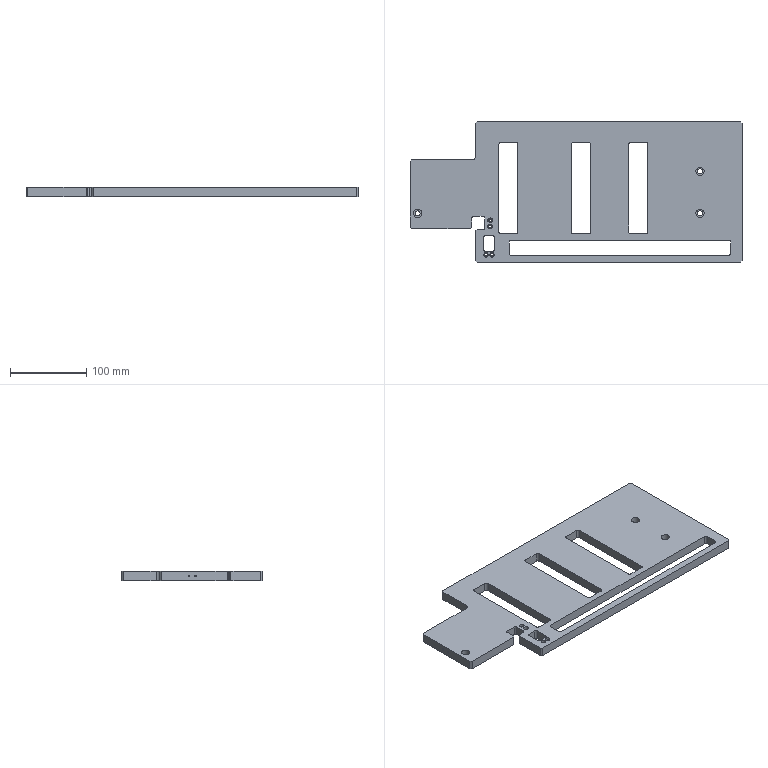NC program | NX | posted with a generic post | part box 435 x 184 x 12 mm
Lines 1793 to 2749 of 10210:
(HOLE_MILLING , TOOL : D6)
N3530 T12 M6
N3532 G54
N3534 G17 G0 G90 X-207.5 Y-28. S9500 M3
N3536 G43 Z30. H12
N3538 Z1.
N3540 G94 G3 X-206.25 Y-29.25 R1.25 F1500.
N3542 X-205. Y-28. R1.25
N3544 X-205. Y-28. Z0.5 I-2.5 J0.
N3546 X-205. Y-28. Z0. I-2.5 J0.
N3548 X-205. Y-28. Z-0.5 I-2.5 J0.
N3550 X-205. Y-28. Z-1. I-2.5 J0.
N3552 X-205. Y-28. Z-1.5 I-2.5 J0.
N3554 X-205. Y-28. Z-2. I-2.5 J0.
N3556 X-205. Y-28. Z-2.5 I-2.5 J0.
N3558 X-205. Y-28. Z-3. I-2.5 J0.
N3560 X-205. Y-28. Z-3.5 I-2.5 J0.
N3562 X-205. Y-28. Z-4. I-2.5 J0.
N3564 X-205. Y-28. Z-4.5 I-2.5 J0.
N3566 X-205. Y-28. Z-5. I-2.5 J0.
N3568 X-205. Y-28. Z-5.5 I-2.5 J0.
N3570 X-205. Y-28. Z-6. I-2.5 J0.
N3572 X-205. Y-28. Z-6.5 I-2.5 J0.
N3574 X-205. Y-28. Z-7. I-2.5 J0.
N3576 X-207.5 Y-25.5 R2.5
N3578 X-205. Y-28. R-2.5
N3580 X-206.25 Y-26.75 R1.25
N3582 X-207.5 Y-28. R1.25
N3584 G0 Z30.
N3586 X162.5
N3588 Z1.
N3590 G3 X163.75 Y-29.25 R1.25
N3592 X165. Y-28. R1.25
N3594 X165. Y-28. Z0.5 I-2.5 J0.
N3596 X165. Y-28. Z0. I-2.5 J0.
N3598 X165. Y-28. Z-0.5 I-2.5 J0.
N3600 X165. Y-28. Z-1. I-2.5 J0.
N3602 X165. Y-28. Z-1.5 I-2.5 J0.
N3604 X165. Y-28. Z-2. I-2.5 J0.
N3606 X165. Y-28. Z-2.5 I-2.5 J0.
N3608 X165. Y-28. Z-3. I-2.5 J0.
N3610 X165. Y-28. Z-3.5 I-2.5 J0.
N3612 X165. Y-28. Z-4. I-2.5 J0.
N3614 X165. Y-28. Z-4.5 I-2.5 J0.
N3616 X165. Y-28. Z-5. I-2.5 J0.
N3618 X165. Y-28. Z-5.5 I-2.5 J0.
N3620 X165. Y-28. Z-6. I-2.5 J0.
N3622 X165. Y-28. Z-6.5 I-2.5 J0.
N3624 X165. Y-28. Z-7. I-2.5 J0.
N3626 X162.5 Y-25.5 R2.5
N3628 X165. Y-28. R-2.5
N3630 X163.75 Y-26.75 R1.25
N3632 X162.5 Y-28. R1.25
N3634 G0 Z30.
N3636 Y27.
N3638 Z1.
N3640 G3 X163.75 Y25.75 R1.25
N3642 X165. Y27. R1.25
N3644 X165. Y27. Z0.5 I-2.5 J0.
N3646 X165. Y27. Z0. I-2.5 J0.
N3648 X165. Y27. Z-0.5 I-2.5 J0.
N3650 X165. Y27. Z-1. I-2.5 J0.
N3652 X165. Y27. Z-1.5 I-2.5 J0.
N3654 X165. Y27. Z-2. I-2.5 J0.
N3656 X165. Y27. Z-2.5 I-2.5 J0.
N3658 X165. Y27. Z-3. I-2.5 J0.
N3660 X165. Y27. Z-3.5 I-2.5 J0.
N3662 X165. Y27. Z-4. I-2.5 J0.
N3664 X165. Y27. Z-4.5 I-2.5 J0.
N3666 X165. Y27. Z-5. I-2.5 J0.
N3668 X165. Y27. Z-5.5 I-2.5 J0.
N3670 X165. Y27. Z-6. I-2.5 J0.
N3672 X165. Y27. Z-6.5 I-2.5 J0.
N3674 X165. Y27. Z-7. I-2.5 J0.
N3676 X162.5 Y29.5 R2.5
N3678 X165. Y27. R-2.5
N3680 X163.75 Y28.25 R1.25
N3682 X162.5 Y27. R1.25
N3684 G0 Z30.
(ZLEVEL_PROFILE_COPY_1_COPY_COPY_1_COPY_COPY_COPY_1 , TOOL : D6)
N3686 X87.957 Y-50.8
N3688 Z-0.5
N3690 G1 X88.477 Y-51.7 F1000.
N3692 G3 X88.996 Y-52. R0.6
N3694 G1 X91. F1500.
N3696 Y-49.996
N3698 G3 X90.7 Y-49.477 R0.6
N3700 G1 X89.8 Y-48.957
N3702 G0 X87.957 Y-50.8 Z-1.
N3704 G1 X88.477 Y-51.7 F1000.
N3706 G3 X88.996 Y-52. R0.6
N3708 G1 X91. F1500.
N3710 Y-49.996
N3712 G3 X90.7 Y-49.477 R0.6
N3714 G1 X89.8 Y-48.957
N3716 G0 X87.957 Y-50.8 Z-1.5
N3718 G1 X88.477 Y-51.7 F1000.
N3720 G3 X88.996 Y-52. R0.6
N3722 G1 X91. F1500.
N3724 Y-49.996
N3726 G3 X90.7 Y-49.477 R0.6
N3728 G1 X89.8 Y-48.957
N3730 G0 X87.957 Y-50.8 Z-2.
N3732 G1 X88.477 Y-51.7 F1000.
N3734 G3 X88.996 Y-52. R0.6
N3736 G1 X91. F1500.
N3738 Y-49.996
N3740 G3 X90.7 Y-49.477 R0.6
N3742 G1 X89.8 Y-48.957
N3744 G0 X87.957 Y-50.8 Z-2.5
N3746 G1 X88.477 Y-51.7 F1000.
N3748 G3 X88.996 Y-52. R0.6
N3750 G1 X91. F1500.
N3752 Y-49.996
N3754 G3 X90.7 Y-49.477 R0.6
N3756 G1 X89.8 Y-48.957
N3758 G0 X87.957 Y-50.8 Z-3.
N3760 G1 X88.477 Y-51.7 F1000.
N3762 G3 X88.996 Y-52. R0.6
N3764 G1 X91. F1500.
N3766 Y-49.996
N3768 G3 X90.7 Y-49.477 R0.6
N3770 G1 X89.8 Y-48.957
N3772 G0 X87.957 Y-50.8 Z-3.5
N3774 G1 X88.477 Y-51.7 F1000.
N3776 G3 X88.996 Y-52. R0.6
N3778 G1 X91. F1500.
N3780 Y-49.996
N3782 G3 X90.7 Y-49.477 R0.6
N3784 G1 X89.8 Y-48.957
N3786 G0 X87.957 Y-50.8 Z-4.
N3788 G1 X88.477 Y-51.7 F1000.
N3790 G3 X88.996 Y-52. R0.6
N3792 G1 X91. F1500.
N3794 Y-49.996
N3796 G3 X90.7 Y-49.477 R0.6
N3798 G1 X89.8 Y-48.957
N3800 G0 X87.957 Y-50.8 Z-4.5
N3802 G1 X88.477 Y-51.7 F1000.
N3804 G3 X88.996 Y-52. R0.6
N3806 G1 X91. F1500.
N3808 Y-49.996
N3810 G3 X90.7 Y-49.477 R0.6
N3812 G1 X89.8 Y-48.957
N3814 G0 X87.957 Y-50.8 Z-5.
N3816 G1 X88.477 Y-51.7 F1000.
N3818 G3 X88.996 Y-52. R0.6
N3820 G1 X91. F1500.
N3822 Y-49.996
N3824 G3 X90.7 Y-49.477 R0.6
N3826 G1 X89.8 Y-48.957
N3828 G0 X87.957 Y-50.8 Z-5.5
N3830 G1 X88.477 Y-51.7 F1000.
N3832 G3 X88.996 Y-52. R0.6
N3834 G1 X91. F1500.
N3836 Y-49.996
N3838 G3 X90.7 Y-49.477 R0.6
N3840 G1 X89.8 Y-48.957
N3842 G0 X87.957 Y-50.8 Z-6.
N3844 G1 X88.477 Y-51.7 F1000.
N3846 G3 X88.996 Y-52. R0.6
N3848 G1 X91. F1500.
N3850 Y-49.996
N3852 G3 X90.7 Y-49.477 R0.6
N3854 G1 X89.8 Y-48.957
N3856 G0 X87.957 Y-50.8 Z-6.5
N3858 G1 X88.477 Y-51.7 F1000.
N3860 G3 X88.996 Y-52. R0.6
N3862 G1 X91. F1500.
N3864 Y-49.996
N3866 G3 X90.7 Y-49.477 R0.6
N3868 G1 X89.8 Y-48.957
N3870 G0 X87.957 Y-50.8 Z-7.
N3872 G1 X88.477 Y-51.7 F1000.
N3874 G3 X88.996 Y-52. R0.6
N3876 G1 X91. F1500.
N3878 Y-49.996
N3880 G3 X90.7 Y-49.477 R0.6
N3882 G1 X89.8 Y-48.957
N3884 G0 X87.957 Y-50.8 Z-7.5
N3886 G1 X88.477 Y-51.7 F1000.
N3888 G3 X88.996 Y-52. R0.6
N3890 G1 X91. F1500.
N3892 Y-49.996
N3894 G3 X90.7 Y-49.477 R0.6
N3896 G1 X89.8 Y-48.957
N3898 G0 X87.957 Y-50.8 Z-8.
N3900 G1 X88.477 Y-51.7 F1000.
N3902 G3 X88.996 Y-52. R0.6
N3904 G1 X91. F1500.
N3906 Y-49.996
N3908 G3 X90.7 Y-49.477 R0.6
N3910 G1 X89.8 Y-48.957
N3912 G0 X87.957 Y-50.8 Z-8.5
N3914 G1 X88.477 Y-51.7 F1000.
N3916 G3 X88.996 Y-52. R0.6
N3918 G1 X91. F1500.
N3920 Y-49.996
N3922 G3 X90.7 Y-49.477 R0.6
N3924 G1 X89.8 Y-48.957
N3926 G0 X87.957 Y-50.8 Z-9.
N3928 G1 X88.477 Y-51.7 F1000.
N3930 G3 X88.996 Y-52. R0.6
N3932 G1 X91. F1500.
N3934 Y-49.996
N3936 G3 X90.7 Y-49.477 R0.6
N3938 G1 X89.8 Y-48.957
N3940 G0 X87.957 Y-50.8 Z-9.5
N3942 G1 X88.477 Y-51.7 F1000.
N3944 G3 X88.996 Y-52. R0.6
N3946 G1 X91. F1500.
N3948 Y-49.996
N3950 G3 X90.7 Y-49.477 R0.6
N3952 G1 X89.8 Y-48.957
N3954 G0 X87.957 Y-50.8 Z-10.
N3956 G1 X88.477 Y-51.7 F1000.
N3958 G3 X88.996 Y-52. R0.6
N3960 G1 X91. F1500.
N3962 Y-49.996
N3964 G3 X90.7 Y-49.477 R0.6
N3966 G1 X89.8 Y-48.957
N3968 G0 X87.957 Y-50.8 Z-10.5
N3970 G1 X88.477 Y-51.7 F1000.
N3972 G3 X88.996 Y-52. R0.6
N3974 G1 X91. F1500.
N3976 Y-49.996
N3978 G3 X90.7 Y-49.477 R0.6
N3980 G1 X89.8 Y-48.957
N3982 G0 X87.957 Y-50.8 Z-11.
N3984 G1 X88.477 Y-51.7 F1000.
N3986 G3 X88.996 Y-52. R0.6
N3988 G1 X91. F1500.
N3990 Y-49.996
N3992 G3 X90.7 Y-49.477 R0.6
N3994 G1 X89.8 Y-48.957
N3996 G0 X87.957 Y-50.8 Z-11.5
N3998 G1 X88.477 Y-51.7 F1000.
N4000 G3 X88.996 Y-52. R0.6
N4002 G1 X91. F1500.
N4004 Y-49.996
N4006 G3 X90.7 Y-49.477 R0.6
N4008 G1 X89.8 Y-48.957
N4010 G0 X87.957 Y-50.8 Z-12.
N4012 G1 X88.477 Y-51.7 F1000.
N4014 G3 X88.996 Y-52. R0.6
N4016 G1 X91. F1500.
N4018 Y-49.996
N4020 G3 X90.7 Y-49.477 R0.6
N4022 G1 X89.8 Y-48.957
N4024 G0 Z30.
N4026 Y58.956
N4028 Z-0.5
N4030 G1 X90.7 Y59.476 F1000.
N4032 G3 X91. Y59.996 R0.6
N4034 G1 Y62. F1500.
N4036 X88.996
N4038 G3 X88.476 Y61.7 R0.6
N4040 G1 X87.956 Y60.8
N4042 G0 X89.8 Y58.956 Z-1.
N4044 G1 X90.7 Y59.476 F1000.
N4046 G3 X91. Y59.996 R0.6
N4048 G1 Y62. F1500.
N4050 X88.996
N4052 G3 X88.476 Y61.7 R0.6
N4054 G1 X87.956 Y60.8
N4056 G0 X89.8 Y58.956 Z-1.5
N4058 G1 X90.7 Y59.476 F1000.
N4060 G3 X91. Y59.996 R0.6
N4062 G1 Y62. F1500.
N4064 X88.996
N4066 G3 X88.476 Y61.7 R0.6
N4068 G1 X87.956 Y60.8
N4070 G0 X89.8 Y58.956 Z-2.
N4072 G1 X90.7 Y59.476 F1000.
N4074 G3 X91. Y59.996 R0.6
N4076 G1 Y62. F1500.
N4078 X88.996
N4080 G3 X88.476 Y61.7 R0.6
N4082 G1 X87.956 Y60.8
N4084 G0 X89.8 Y58.956 Z-2.5
N4086 G1 X90.7 Y59.476 F1000.
N4088 G3 X91. Y59.996 R0.6
N4090 G1 Y62. F1500.
N4092 X88.996
N4094 G3 X88.476 Y61.7 R0.6
N4096 G1 X87.956 Y60.8
N4098 G0 X89.8 Y58.956 Z-3.
N4100 G1 X90.7 Y59.476 F1000.
N4102 G3 X91. Y59.996 R0.6
N4104 G1 Y62. F1500.
N4106 X88.996
N4108 G3 X88.476 Y61.7 R0.6
N4110 G1 X87.956 Y60.8
N4112 G0 X89.8 Y58.956 Z-3.5
N4114 G1 X90.7 Y59.476 F1000.
N4116 G3 X91. Y59.996 R0.6
N4118 G1 Y62. F1500.
N4120 X88.996
N4122 G3 X88.476 Y61.7 R0.6
N4124 G1 X87.956 Y60.8
N4126 G0 X89.8 Y58.956 Z-4.
N4128 G1 X90.7 Y59.476 F1000.
N4130 G3 X91. Y59.996 R0.6
N4132 G1 Y62. F1500.
N4134 X88.996
N4136 G3 X88.476 Y61.7 R0.6
N4138 G1 X87.956 Y60.8
N4140 G0 X89.8 Y58.956 Z-4.5
N4142 G1 X90.7 Y59.476 F1000.
N4144 G3 X91. Y59.996 R0.6
N4146 G1 Y62. F1500.
N4148 X88.996
N4150 G3 X88.476 Y61.7 R0.6
N4152 G1 X87.956 Y60.8
N4154 G0 X89.8 Y58.956 Z-5.
N4156 G1 X90.7 Y59.476 F1000.
N4158 G3 X91. Y59.996 R0.6
N4160 G1 Y62. F1500.
N4162 X88.996
N4164 G3 X88.476 Y61.7 R0.6
N4166 G1 X87.956 Y60.8
N4168 G0 X89.8 Y58.956 Z-5.5
N4170 G1 X90.7 Y59.476 F1000.
N4172 G3 X91. Y59.996 R0.6
N4174 G1 Y62. F1500.
N4176 X88.996
N4178 G3 X88.476 Y61.7 R0.6
N4180 G1 X87.956 Y60.8
N4182 G0 X89.8 Y58.956 Z-6.
N4184 G1 X90.7 Y59.476 F1000.
N4186 G3 X91. Y59.996 R0.6
N4188 G1 Y62. F1500.
N4190 X88.996
N4192 G3 X88.476 Y61.7 R0.6
N4194 G1 X87.956 Y60.8
N4196 G0 X89.8 Y58.956 Z-6.5
N4198 G1 X90.7 Y59.476 F1000.
N4200 G3 X91. Y59.996 R0.6
N4202 G1 Y62. F1500.
N4204 X88.996
N4206 G3 X88.476 Y61.7 R0.6
N4208 G1 X87.956 Y60.8
N4210 G0 X89.8 Y58.956 Z-7.
N4212 G1 X90.7 Y59.476 F1000.
N4214 G3 X91. Y59.996 R0.6
N4216 G1 Y62. F1500.
N4218 X88.996
N4220 G3 X88.476 Y61.7 R0.6
N4222 G1 X87.956 Y60.8
N4224 G0 X89.8 Y58.956 Z-7.5
N4226 G1 X90.7 Y59.476 F1000.
N4228 G3 X91. Y59.996 R0.6
N4230 G1 Y62. F1500.
N4232 X88.996
N4234 G3 X88.476 Y61.7 R0.6
N4236 G1 X87.956 Y60.8
N4238 G0 X89.8 Y58.956 Z-8.
N4240 G1 X90.7 Y59.476 F1000.
N4242 G3 X91. Y59.996 R0.6
N4244 G1 Y62. F1500.
N4246 X88.996
N4248 G3 X88.476 Y61.7 R0.6
N4250 G1 X87.956 Y60.8
N4252 G0 X89.8 Y58.956 Z-8.5
N4254 G1 X90.7 Y59.476 F1000.
N4256 G3 X91. Y59.996 R0.6
N4258 G1 Y62. F1500.
N4260 X88.996
N4262 G3 X88.476 Y61.7 R0.6
N4264 G1 X87.956 Y60.8
N4266 G0 X89.8 Y58.956 Z-9.
N4268 G1 X90.7 Y59.476 F1000.
N4270 G3 X91. Y59.996 R0.6
N4272 G1 Y62. F1500.
N4274 X88.996
N4276 G3 X88.476 Y61.7 R0.6
N4278 G1 X87.956 Y60.8
N4280 G0 X89.8 Y58.956 Z-9.5
N4282 G1 X90.7 Y59.476 F1000.
N4284 G3 X91. Y59.996 R0.6
N4286 G1 Y62. F1500.
N4288 X88.996
N4290 G3 X88.476 Y61.7 R0.6
N4292 G1 X87.956 Y60.8
N4294 G0 X89.8 Y58.956 Z-10.
N4296 G1 X90.7 Y59.476 F1000.
N4298 G3 X91. Y59.996 R0.6
N4300 G1 Y62. F1500.
N4302 X88.996
N4304 G3 X88.476 Y61.7 R0.6
N4306 G1 X87.956 Y60.8
N4308 G0 X89.8 Y58.956 Z-10.5
N4310 G1 X90.7 Y59.476 F1000.
N4312 G3 X91. Y59.996 R0.6
N4314 G1 Y62. F1500.
N4316 X88.996
N4318 G3 X88.476 Y61.7 R0.6
N4320 G1 X87.956 Y60.8
N4322 G0 X89.8 Y58.956 Z-11.
N4324 G1 X90.7 Y59.476 F1000.
N4326 G3 X91. Y59.996 R0.6
N4328 G1 Y62. F1500.
N4330 X88.996
N4332 G3 X88.476 Y61.7 R0.6
N4334 G1 X87.956 Y60.8
N4336 G0 X89.8 Y58.956 Z-11.5
N4338 G1 X90.7 Y59.476 F1000.
N4340 G3 X91. Y59.996 R0.6
N4342 G1 Y62. F1500.
N4344 X88.996
N4346 G3 X88.476 Y61.7 R0.6
N4348 G1 X87.956 Y60.8
N4350 G0 X89.8 Y58.956 Z-12.
N4352 G1 X90.7 Y59.476 F1000.
N4354 G3 X91. Y59.996 R0.6
N4356 G1 Y62. F1500.
N4358 X88.996
N4360 G3 X88.476 Y61.7 R0.6
N4362 G1 X87.956 Y60.8
N4364 G0 Z30.
N4366 X75.045
N4368 Z-0.5
N4370 G1 X74.526 Y61.7 F1000.
N4372 G3 X74.006 Y62. R0.6
N4374 G1 X72. F1500.
N4376 Y59.994
N4378 G3 X72.3 Y59.474 R0.6
N4380 G1 X73.2 Y58.955
N4382 G0 X75.045 Y60.8 Z-1.
N4384 G1 X74.526 Y61.7 F1000.
N4386 G3 X74.006 Y62. R0.6
N4388 G1 X72. F1500.
N4390 Y59.994
N4392 G3 X72.3 Y59.474 R0.6
N4394 G1 X73.2 Y58.955
N4396 G0 X75.045 Y60.8 Z-1.5
N4398 G1 X74.526 Y61.7 F1000.
N4400 G3 X74.006 Y62. R0.6
N4402 G1 X72. F1500.
N4404 Y59.994
N4406 G3 X72.3 Y59.474 R0.6
N4408 G1 X73.2 Y58.955
N4410 G0 X75.045 Y60.8 Z-2.
N4412 G1 X74.526 Y61.7 F1000.
N4414 G3 X74.006 Y62. R0.6
N4416 G1 X72. F1500.
N4418 Y59.994
N4420 G3 X72.3 Y59.474 R0.6
N4422 G1 X73.2 Y58.955
N4424 G0 X75.045 Y60.8 Z-2.5
N4426 G1 X74.526 Y61.7 F1000.
N4428 G3 X74.006 Y62. R0.6
N4430 G1 X72. F1500.
N4432 Y59.994
N4434 G3 X72.3 Y59.474 R0.6
N4436 G1 X73.2 Y58.955
N4438 G0 X75.045 Y60.8 Z-3.
N4440 G1 X74.526 Y61.7 F1000.
N4442 G3 X74.006 Y62. R0.6
N4444 G1 X72. F1500.
N4446 Y59.994
N4448 G3 X72.3 Y59.474 R0.6
N4450 G1 X73.2 Y58.955
N4452 G0 X75.045 Y60.8 Z-3.5
N4454 G1 X74.526 Y61.7 F1000.
N4456 G3 X74.006 Y62. R0.6
N4458 G1 X72. F1500.
N4460 Y59.994
N4462 G3 X72.3 Y59.474 R0.6
N4464 G1 X73.2 Y58.955
N4466 G0 X75.045 Y60.8 Z-4.
N4468 G1 X74.526 Y61.7 F1000.
N4470 G3 X74.006 Y62. R0.6
N4472 G1 X72. F1500.
N4474 Y59.994
N4476 G3 X72.3 Y59.474 R0.6
N4478 G1 X73.2 Y58.955
N4480 G0 X75.045 Y60.8 Z-4.5
N4482 G1 X74.526 Y61.7 F1000.
N4484 G3 X74.006 Y62. R0.6
N4486 G1 X72. F1500.
N4488 Y59.994
N4490 G3 X72.3 Y59.474 R0.6
N4492 G1 X73.2 Y58.955
N4494 G0 X75.045 Y60.8 Z-5.
N4496 G1 X74.526 Y61.7 F1000.
N4498 G3 X74.006 Y62. R0.6
N4500 G1 X72. F1500.
N4502 Y59.994
N4504 G3 X72.3 Y59.474 R0.6
N4506 G1 X73.2 Y58.955
N4508 G0 X75.045 Y60.8 Z-5.5
N4510 G1 X74.526 Y61.7 F1000.
N4512 G3 X74.006 Y62. R0.6
N4514 G1 X72. F1500.
N4516 Y59.994
N4518 G3 X72.3 Y59.474 R0.6
N4520 G1 X73.2 Y58.955
N4522 G0 X75.045 Y60.8 Z-6.
N4524 G1 X74.526 Y61.7 F1000.
N4526 G3 X74.006 Y62. R0.6
N4528 G1 X72. F1500.
N4530 Y59.994
N4532 G3 X72.3 Y59.474 R0.6
N4534 G1 X73.2 Y58.955
N4536 G0 X75.045 Y60.8 Z-6.5
N4538 G1 X74.526 Y61.7 F1000.
N4540 G3 X74.006 Y62. R0.6
N4542 G1 X72. F1500.
N4544 Y59.994
N4546 G3 X72.3 Y59.474 R0.6
N4548 G1 X73.2 Y58.955
N4550 G0 X75.045 Y60.8 Z-7.
N4552 G1 X74.526 Y61.7 F1000.
N4554 G3 X74.006 Y62. R0.6
N4556 G1 X72. F1500.
N4558 Y59.994
N4560 G3 X72.3 Y59.474 R0.6
N4562 G1 X73.2 Y58.955
N4564 G0 X75.045 Y60.8 Z-7.5
N4566 G1 X74.526 Y61.7 F1000.
N4568 G3 X74.006 Y62. R0.6
N4570 G1 X72. F1500.
N4572 Y59.994
N4574 G3 X72.3 Y59.474 R0.6
N4576 G1 X73.2 Y58.955
N4578 G0 X75.045 Y60.8 Z-8.
N4580 G1 X74.526 Y61.7 F1000.
N4582 G3 X74.006 Y62. R0.6
N4584 G1 X72. F1500.
N4586 Y59.994
N4588 G3 X72.3 Y59.474 R0.6
N4590 G1 X73.2 Y58.955
N4592 G0 X75.045 Y60.8 Z-8.5
N4594 G1 X74.526 Y61.7 F1000.
N4596 G3 X74.006 Y62. R0.6
N4598 G1 X72. F1500.
N4600 Y59.994
N4602 G3 X72.3 Y59.474 R0.6
N4604 G1 X73.2 Y58.955
N4606 G0 X75.045 Y60.8 Z-9.
N4608 G1 X74.526 Y61.7 F1000.
N4610 G3 X74.006 Y62. R0.6
N4612 G1 X72. F1500.
N4614 Y59.994
N4616 G3 X72.3 Y59.474 R0.6
N4618 G1 X73.2 Y58.955
N4620 G0 X75.045 Y60.8 Z-9.5
N4622 G1 X74.526 Y61.7 F1000.
N4624 G3 X74.006 Y62. R0.6
N4626 G1 X72. F1500.
N4628 Y59.994
N4630 G3 X72.3 Y59.474 R0.6
N4632 G1 X73.2 Y58.955
N4634 G0 X75.045 Y60.8 Z-10.
N4636 G1 X74.526 Y61.7 F1000.
N4638 G3 X74.006 Y62. R0.6
N4640 G1 X72. F1500.
N4642 Y59.994
N4644 G3 X72.3 Y59.474 R0.6
N4646 G1 X73.2 Y58.955
N4648 G0 X75.045 Y60.8 Z-10.5
N4650 G1 X74.526 Y61.7 F1000.
N4652 G3 X74.006 Y62. R0.6
N4654 G1 X72. F1500.
N4656 Y59.994
N4658 G3 X72.3 Y59.474 R0.6
N4660 G1 X73.2 Y58.955
N4662 G0 X75.045 Y60.8 Z-11.
N4664 G1 X74.526 Y61.7 F1000.
N4666 G3 X74.006 Y62. R0.6
N4668 G1 X72. F1500.
N4670 Y59.994
N4672 G3 X72.3 Y59.474 R0.6
N4674 G1 X73.2 Y58.955
N4676 G0 X75.045 Y60.8 Z-11.5
N4678 G1 X74.526 Y61.7 F1000.
N4680 G3 X74.006 Y62. R0.6
N4682 G1 X72. F1500.
N4684 Y59.994
N4686 G3 X72.3 Y59.474 R0.6
N4688 G1 X73.2 Y58.955
N4690 G0 X75.045 Y60.8 Z-12.
N4692 G1 X74.526 Y61.7 F1000.
N4694 G3 X74.006 Y62. R0.6
N4696 G1 X72. F1500.
N4698 Y59.994
N4700 G3 X72.3 Y59.474 R0.6
N4702 G1 X73.2 Y58.955
N4704 G0 Z30.
N4706 Y-48.954
N4708 Z-0.5
N4710 G1 X72.3 Y-49.474 F1000.
N4712 G3 X72. Y-49.994 R0.6
N4714 G1 Y-52. F1500.
N4716 X74.006
N4718 G3 X74.526 Y-51.7 R0.6
N4720 G1 X75.046 Y-50.8
N4722 G0 X73.2 Y-48.954 Z-1.
N4724 G1 X72.3 Y-49.474 F1000.
N4726 G3 X72. Y-49.994 R0.6
N4728 G1 Y-52. F1500.
N4730 X74.006
N4732 G3 X74.526 Y-51.7 R0.6
N4734 G1 X75.046 Y-50.8
N4736 G0 X73.2 Y-48.954 Z-1.5
N4738 G1 X72.3 Y-49.474 F1000.
N4740 G3 X72. Y-49.994 R0.6
N4742 G1 Y-52. F1500.
N4744 X74.006
N4746 G3 X74.526 Y-51.7 R0.6
N4748 G1 X75.046 Y-50.8
N4750 G0 X73.2 Y-48.954 Z-2.
N4752 G1 X72.3 Y-49.474 F1000.
N4754 G3 X72. Y-49.994 R0.6
N4756 G1 Y-52. F1500.
N4758 X74.006
N4760 G3 X74.526 Y-51.7 R0.6
N4762 G1 X75.046 Y-50.8
N4764 G0 X73.2 Y-48.954 Z-2.5
N4766 G1 X72.3 Y-49.474 F1000.
N4768 G3 X72. Y-49.994 R0.6
N4770 G1 Y-52. F1500.
N4772 X74.006
N4774 G3 X74.526 Y-51.7 R0.6
N4776 G1 X75.046 Y-50.8
N4778 G0 X73.2 Y-48.954 Z-3.
N4780 G1 X72.3 Y-49.474 F1000.
N4782 G3 X72. Y-49.994 R0.6
N4784 G1 Y-52. F1500.
N4786 X74.006
N4788 G3 X74.526 Y-51.7 R0.6
N4790 G1 X75.046 Y-50.8
N4792 G0 X73.2 Y-48.954 Z-3.5
N4794 G1 X72.3 Y-49.474 F1000.
N4796 G3 X72. Y-49.994 R0.6
N4798 G1 Y-52. F1500.
N4800 X74.006
N4802 G3 X74.526 Y-51.7 R0.6
N4804 G1 X75.046 Y-50.8
N4806 G0 X73.2 Y-48.954 Z-4.
N4808 G1 X72.3 Y-49.474 F1000.
N4810 G3 X72. Y-49.994 R0.6
N4812 G1 Y-52. F1500.
N4814 X74.006
N4816 G3 X74.526 Y-51.7 R0.6
N4818 G1 X75.046 Y-50.8
N4820 G0 X73.2 Y-48.954 Z-4.5
N4822 G1 X72.3 Y-49.474 F1000.
N4824 G3 X72. Y-49.994 R0.6
N4826 G1 Y-52. F1500.
N4828 X74.006
N4830 G3 X74.526 Y-51.7 R0.6
N4832 G1 X75.046 Y-50.8
N4834 G0 X73.2 Y-48.954 Z-5.
N4836 G1 X72.3 Y-49.474 F1000.
N4838 G3 X72. Y-49.994 R0.6
N4840 G1 Y-52. F1500.
N4842 X74.006
N4844 G3 X74.526 Y-51.7 R0.6
N4846 G1 X75.046 Y-50.8
N4848 G0 X73.2 Y-48.954 Z-5.5
N4850 G1 X72.3 Y-49.474 F1000.
N4852 G3 X72. Y-49.994 R0.6
N4854 G1 Y-52. F1500.
N4856 X74.006
N4858 G3 X74.526 Y-51.7 R0.6
N4860 G1 X75.046 Y-50.8
N4862 G0 X73.2 Y-48.954 Z-6.
N4864 G1 X72.3 Y-49.474 F1000.
N4866 G3 X72. Y-49.994 R0.6
N4868 G1 Y-52. F1500.
N4870 X74.006
N4872 G3 X74.526 Y-51.7 R0.6
N4874 G1 X75.046 Y-50.8
N4876 G0 X73.2 Y-48.954 Z-6.5
N4878 G1 X72.3 Y-49.474 F1000.
N4880 G3 X72. Y-49.994 R0.6
N4882 G1 Y-52. F1500.
N4884 X74.006
N4886 G3 X74.526 Y-51.7 R0.6
N4888 G1 X75.046 Y-50.8
N4890 G0 X73.2 Y-48.954 Z-7.
N4892 G1 X72.3 Y-49.474 F1000.
N4894 G3 X72. Y-49.994 R0.6
N4896 G1 Y-52. F1500.
N4898 X74.006
N4900 G3 X74.526 Y-51.7 R0.6
N4902 G1 X75.046 Y-50.8
N4904 G0 X73.2 Y-48.954 Z-7.5
N4906 G1 X72.3 Y-49.474 F1000.
N4908 G3 X72. Y-49.994 R0.6
N4910 G1 Y-52. F1500.
N4912 X74.006
N4914 G3 X74.526 Y-51.7 R0.6
N4916 G1 X75.046 Y-50.8
N4918 G0 X73.2 Y-48.954 Z-8.
N4920 G1 X72.3 Y-49.474 F1000.
N4922 G3 X72. Y-49.994 R0.6
N4924 G1 Y-52. F1500.
N4926 X74.006
N4928 G3 X74.526 Y-51.7 R0.6
N4930 G1 X75.046 Y-50.8
N4932 G0 X73.2 Y-48.954 Z-8.5
N4934 G1 X72.3 Y-49.474 F1000.
N4936 G3 X72. Y-49.994 R0.6
N4938 G1 Y-52. F1500.
N4940 X74.006
N4942 G3 X74.526 Y-51.7 R0.6
N4944 G1 X75.046 Y-50.8
N4946 G0 X73.2 Y-48.954 Z-9.
N4948 G1 X72.3 Y-49.474 F1000.
N4950 G3 X72. Y-49.994 R0.6
N4952 G1 Y-52. F1500.
N4954 X74.006
N4956 G3 X74.526 Y-51.7 R0.6
N4958 G1 X75.046 Y-50.8
N4960 G0 X73.2 Y-48.954 Z-9.5
N4962 G1 X72.3 Y-49.474 F1000.
N4964 G3 X72. Y-49.994 R0.6
N4966 G1 Y-52. F1500.
N4968 X74.006
N4970 G3 X74.526 Y-51.7 R0.6
N4972 G1 X75.046 Y-50.8
N4974 G0 X73.2 Y-48.954 Z-10.
N4976 G1 X72.3 Y-49.474 F1000.
N4978 G3 X72. Y-49.994 R0.6
N4980 G1 Y-52. F1500.
N4982 X74.006
N4984 G3 X74.526 Y-51.7 R0.6
N4986 G1 X75.046 Y-50.8
N4988 G0 X73.2 Y-48.954 Z-10.5
N4990 G1 X72.3 Y-49.474 F1000.
N4992 G3 X72. Y-49.994 R0.6
N4994 G1 Y-52. F1500.
N4996 X74.006
N4998 G3 X74.526 Y-51.7 R0.6
N5000 G1 X75.046 Y-50.8
N5002 G0 X73.2 Y-48.954 Z-11.
N5004 G1 X72.3 Y-49.474 F1000.
N5006 G3 X72. Y-49.994 R0.6
N5008 G1 Y-52. F1500.
N5010 X74.006
N5012 G3 X74.526 Y-51.7 R0.6
N5014 G1 X75.046 Y-50.8
N5016 G0 X73.2 Y-48.954 Z-11.5
N5018 G1 X72.3 Y-49.474 F1000.
N5020 G3 X72. Y-49.994 R0.6
N5022 G1 Y-52. F1500.
N5024 X74.006
N5026 G3 X74.526 Y-51.7 R0.6
N5028 G1 X75.046 Y-50.8
N5030 G0 X73.2 Y-48.954 Z-12.
N5032 G1 X72.3 Y-49.474 F1000.
N5034 G3 X72. Y-49.994 R0.6
N5036 G1 Y-52. F1500.
N5038 X74.006
N5040 G3 X74.526 Y-51.7 R0.6
N5042 G1 X75.046 Y-50.8
N5044 G0 Z53.
N5046 X12.956
N5048 Z-0.5
N5050 G1 X13.476 Y-51.7 F1000.
N5052 G3 X13.996 Y-52. R0.6
N5054 G1 X16. F1500.
N5056 Y-49.996
N5058 G3 X15.7 Y-49.476 R0.6
N5060 G1 X14.8 Y-48.956
N5062 G0 X12.956 Y-50.8 Z-1.
N5064 G1 X13.476 Y-51.7 F1000.
N5066 G3 X13.996 Y-52. R0.6
N5068 G1 X16. F1500.
N5070 Y-49.996
N5072 G3 X15.7 Y-49.476 R0.6
N5074 G1 X14.8 Y-48.956
N5076 G0 X12.956 Y-50.8 Z-1.5
N5078 G1 X13.476 Y-51.7 F1000.
N5080 G3 X13.996 Y-52. R0.6
N5082 G1 X16. F1500.
N5084 Y-49.996
N5086 G3 X15.7 Y-49.476 R0.6
N5088 G1 X14.8 Y-48.956
N5090 G0 X12.956 Y-50.8 Z-2.
N5092 G1 X13.476 Y-51.7 F1000.
N5094 G3 X13.996 Y-52. R0.6
N5096 G1 X16. F1500.
N5098 Y-49.996
N5100 G3 X15.7 Y-49.476 R0.6
N5102 G1 X14.8 Y-48.956
N5104 G0 X12.956 Y-50.8 Z-2.5
N5106 G1 X13.476 Y-51.7 F1000.
N5108 G3 X13.996 Y-52. R0.6
N5110 G1 X16. F1500.
N5112 Y-49.996
N5114 G3 X15.7 Y-49.476 R0.6
N5116 G1 X14.8 Y-48.956
N5118 G0 X12.956 Y-50.8 Z-3.
N5120 G1 X13.476 Y-51.7 F1000.
N5122 G3 X13.996 Y-52. R0.6
N5124 G1 X16. F1500.
N5126 Y-49.996
N5128 G3 X15.7 Y-49.476 R0.6
N5130 G1 X14.8 Y-48.956
N5132 G0 X12.956 Y-50.8 Z-3.5
N5134 G1 X13.476 Y-51.7 F1000.
N5136 G3 X13.996 Y-52. R0.6
N5138 G1 X16. F1500.
N5140 Y-49.996
N5142 G3 X15.7 Y-49.476 R0.6
N5144 G1 X14.8 Y-48.956
N5146 G0 X12.956 Y-50.8 Z-4.
N5148 G1 X13.476 Y-51.7 F1000.
N5150 G3 X13.996 Y-52. R0.6
N5152 G1 X16. F1500.
N5154 Y-49.996
N5156 G3 X15.7 Y-49.476 R0.6
N5158 G1 X14.8 Y-48.956
N5160 G0 X12.956 Y-50.8 Z-4.5
N5162 G1 X13.476 Y-51.7 F1000.
N5164 G3 X13.996 Y-52. R0.6
N5166 G1 X16. F1500.
N5168 Y-49.996
N5170 G3 X15.7 Y-49.476 R0.6
N5172 G1 X14.8 Y-48.956
N5174 G0 X12.956 Y-50.8 Z-5.
N5176 G1 X13.476 Y-51.7 F1000.
N5178 G3 X13.996 Y-52. R0.6
N5180 G1 X16. F1500.
N5182 Y-49.996
N5184 G3 X15.7 Y-49.476 R0.6
N5186 G1 X14.8 Y-48.956
N5188 G0 X12.956 Y-50.8 Z-5.5
N5190 G1 X13.476 Y-51.7 F1000.
N5192 G3 X13.996 Y-52. R0.6
N5194 G1 X16. F1500.
N5196 Y-49.996
N5198 G3 X15.7 Y-49.476 R0.6
N5200 G1 X14.8 Y-48.956
N5202 G0 X12.956 Y-50.8 Z-6.
N5204 G1 X13.476 Y-51.7 F1000.
N5206 G3 X13.996 Y-52. R0.6
N5208 G1 X16. F1500.
N5210 Y-49.996
N5212 G3 X15.7 Y-49.476 R0.6
N5214 G1 X14.8 Y-48.956
N5216 G0 X12.956 Y-50.8 Z-6.5
N5218 G1 X13.476 Y-51.7 F1000.
N5220 G3 X13.996 Y-52. R0.6
N5222 G1 X16. F1500.
N5224 Y-49.996
N5226 G3 X15.7 Y-49.476 R0.6
N5228 G1 X14.8 Y-48.956
N5230 G0 X12.956 Y-50.8 Z-7.
N5232 G1 X13.476 Y-51.7 F1000.
N5234 G3 X13.996 Y-52. R0.6
N5236 G1 X16. F1500.
N5238 Y-49.996
N5240 G3 X15.7 Y-49.476 R0.6
N5242 G1 X14.8 Y-48.956
N5244 G0 X12.956 Y-50.8 Z-7.5
N5246 G1 X13.476 Y-51.7 F1000.
N5248 G3 X13.996 Y-52. R0.6
N5250 G1 X16. F1500.
N5252 Y-49.996
N5254 G3 X15.7 Y-49.476 R0.6
N5256 G1 X14.8 Y-48.956
N5258 G0 X12.956 Y-50.8 Z-8.
N5260 G1 X13.476 Y-51.7 F1000.
N5262 G3 X13.996 Y-52. R0.6
N5264 G1 X16. F1500.
N5266 Y-49.996
N5268 G3 X15.7 Y-49.476 R0.6
N5270 G1 X14.8 Y-48.956
N5272 G0 X12.956 Y-50.8 Z-8.5
N5274 G1 X13.476 Y-51.7 F1000.
N5276 G3 X13.996 Y-52. R0.6
N5278 G1 X16. F1500.
N5280 Y-49.996
N5282 G3 X15.7 Y-49.476 R0.6
N5284 G1 X14.8 Y-48.956
N5286 G0 X12.956 Y-50.8 Z-9.
N5288 G1 X13.476 Y-51.7 F1000.
N5290 G3 X13.996 Y-52. R0.6
N5292 G1 X16. F1500.
N5294 Y-49.996
N5296 G3 X15.7 Y-49.476 R0.6
N5298 G1 X14.8 Y-48.956
N5300 G0 X12.956 Y-50.8 Z-9.5
N5302 G1 X13.476 Y-51.7 F1000.
N5304 G3 X13.996 Y-52. R0.6
N5306 G1 X16. F1500.
N5308 Y-49.996
N5310 G3 X15.7 Y-49.476 R0.6
N5312 G1 X14.8 Y-48.956
N5314 G0 X12.956 Y-50.8 Z-10.
N5316 G1 X13.476 Y-51.7 F1000.
N5318 G3 X13.996 Y-52. R0.6
N5320 G1 X16. F1500.
N5322 Y-49.996
N5324 G3 X15.7 Y-49.476 R0.6
N5326 G1 X14.8 Y-48.956
N5328 G0 X12.956 Y-50.8 Z-10.5
N5330 G1 X13.476 Y-51.7 F1000.
N5332 G3 X13.996 Y-52. R0.6
N5334 G1 X16. F1500.
N5336 Y-49.996
N5338 G3 X15.7 Y-49.476 R0.6
N5340 G1 X14.8 Y-48.956
N5342 G0 X12.956 Y-50.8 Z-11.
N5344 G1 X13.476 Y-51.7 F1000.
N5346 G3 X13.996 Y-52. R0.6
N5348 G1 X16. F1500.
N5350 Y-49.996
N5352 G3 X15.7 Y-49.476 R0.6
N5354 G1 X14.8 Y-48.956
N5356 G0 X12.956 Y-50.8 Z-11.5
N5358 G1 X13.476 Y-51.7 F1000.
N5360 G3 X13.996 Y-52. R0.6
N5362 G1 X16. F1500.
N5364 Y-49.996
N5366 G3 X15.7 Y-49.476 R0.6
N5368 G1 X14.8 Y-48.956
N5370 G0 X12.956 Y-50.8 Z-12.
N5372 G1 X13.476 Y-51.7 F1000.
N5374 G3 X13.996 Y-52. R0.6
N5376 G1 X16. F1500.
N5378 Y-49.996
N5380 G3 X15.7 Y-49.476 R0.6
N5382 G1 X14.8 Y-48.956
N5384 G0 Z30.
N5386 Y58.955
N5388 Z-0.5
N5390 G1 X15.7 Y59.475 F1000.
N5392 G3 X16. Y59.994 R0.6
N5394 G1 Y62. F1500.
N5396 X13.994
N5398 G3 X13.475 Y61.7 R0.6
N5400 G1 X12.955 Y60.8
N5402 G0 X14.8 Y58.955 Z-1.
N5404 G1 X15.7 Y59.475 F1000.
N5406 G3 X16. Y59.994 R0.6
N5408 G1 Y62. F1500.
N5410 X13.994
N5412 G3 X13.475 Y61.7 R0.6
N5414 G1 X12.955 Y60.8
N5416 G0 X14.8 Y58.955 Z-1.5
N5418 G1 X15.7 Y59.475 F1000.
N5420 G3 X16. Y59.994 R0.6
N5422 G1 Y62. F1500.
N5424 X13.994
N5426 G3 X13.475 Y61.7 R0.6
N5428 G1 X12.955 Y60.8
N5430 G0 X14.8 Y58.955 Z-2.